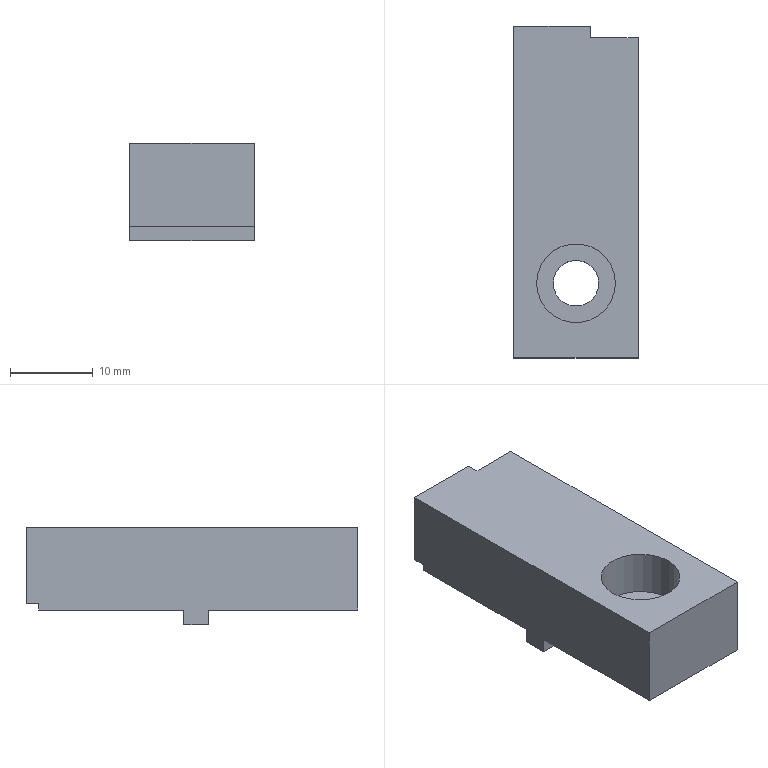Part | STEP file | Rivet push-in slide2_Default | 1 solid | 19 faces | box 15 x 40 x 11.8 mm | volume 5491 mm3 | plane 15 | cylinder 4 | commonest cylinder face diameters 5.5 x2 9.5 x2
STEP:
#1=CARTESIAN_POINT('',(0.,0.,0.));
#2=DIRECTION('',(0.,0.,1.));
#3=DIRECTION('',(1.,0.,0.));
#4=AXIS2_PLACEMENT_3D('',#1,#2,#3);
#5=CARTESIAN_POINT('',(22.25,-1.,4.5));
#6=VERTEX_POINT('',#5);
#7=CARTESIAN_POINT('',(22.25,-1.,10.));
#8=VERTEX_POINT('',#7);
#9=CARTESIAN_POINT('',(22.25,-1.,10.));
#10=DIRECTION('',(0.,0.,1.));
#11=VECTOR('',#10,1.);
#12=LINE('',#9,#11);
#13=CARTESIAN_POINT('',(17.5,-1.,10.));
#14=DIRECTION('',(0.,0.,1.));
#15=DIRECTION('',(1.,0.,0.));
#16=AXIS2_PLACEMENT_3D('',#13,#14,#15);
#17=CYLINDRICAL_SURFACE('',#16,4.75);
#18=CARTESIAN_POINT('',(6.283,0.));
#19=DIRECTION('',(0.,1.));
#20=VECTOR('',#19,1.);
#21=LINE('',#18,#20);
#22=(GEOMETRIC_REPRESENTATION_CONTEXT(2)PARAMETRIC_REPRESENTATION_CONTEXT()REPRESENTATION_CONTEXT('',''));
#23=DEFINITIONAL_REPRESENTATION('',(#21),#22);
#24=PCURVE('',#17,#23);
#25=CARTESIAN_POINT('',(17.5,-1.,10.));
#26=DIRECTION('',(0.,0.,1.));
#27=DIRECTION('',(1.,0.,0.));
#28=AXIS2_PLACEMENT_3D('',#25,#26,#27);
#29=CYLINDRICAL_SURFACE('',#28,4.75);
#30=CARTESIAN_POINT('',(0.,0.));
#31=DIRECTION('',(0.,1.));
#32=VECTOR('',#31,1.);
#33=LINE('',#30,#32);
#34=(GEOMETRIC_REPRESENTATION_CONTEXT(2)PARAMETRIC_REPRESENTATION_CONTEXT()REPRESENTATION_CONTEXT('',''));
#35=DEFINITIONAL_REPRESENTATION('',(#33),#34);
#36=PCURVE('',#29,#35);
#37=SURFACE_CURVE('',#12,(#24,#36),.PCURVE_S1.);
#38=EDGE_CURVE('',#6,#8,#37,.T.);
#39=ORIENTED_EDGE('',*,*,#38,.T.);
#40=CARTESIAN_POINT('',(12.75,-1.,10.));
#41=VERTEX_POINT('',#40);
#42=CARTESIAN_POINT('',(17.5,-1.,10.));
#43=DIRECTION('',(0.,0.,1.));
#44=DIRECTION('',(1.,0.,0.));
#45=AXIS2_PLACEMENT_3D('',#42,#43,#44);
#46=CIRCLE('',#45,4.75);
#47=CARTESIAN_POINT('',(0.,0.));
#48=DIRECTION('',(1.,0.));
#49=VECTOR('',#48,1.);
#50=LINE('',#47,#49);
#51=(GEOMETRIC_REPRESENTATION_CONTEXT(2)PARAMETRIC_REPRESENTATION_CONTEXT()REPRESENTATION_CONTEXT('',''));
#52=DEFINITIONAL_REPRESENTATION('',(#50),#51);
#53=PCURVE('',#17,#52);
#54=CARTESIAN_POINT('',(0.,30.,10.));
#55=DIRECTION('',(0.,0.,-1.));
#56=DIRECTION('',(-1.,0.,0.));
#57=AXIS2_PLACEMENT_3D('',#54,#55,#56);
#58=PLANE('',#57);
#59=CARTESIAN_POINT('',(-22.25,-31.));
#60=CARTESIAN_POINT('',(-22.25,-22.773));
#61=CARTESIAN_POINT('',(-15.125,-26.886));
#62=CARTESIAN_POINT('',(-8.,-31.));
#63=CARTESIAN_POINT('',(-15.125,-35.114));
#64=CARTESIAN_POINT('',(-22.25,-39.227));
#65=CARTESIAN_POINT('',(-22.25,-31.));
#66=(BOUNDED_CURVE()B_SPLINE_CURVE(2,(#59,#60,#61,#62,#63,#64,#65),.UNSPECIFIED.,.T.,.F.)B_SPLINE_CURVE_WITH_KNOTS((1,2,2,2,2,1),(-2.094,0.,2.094,4.189,6.283,8.378),.UNSPECIFIED.)CURVE()GEOMETRIC_REPRESENTATION_ITEM()RATIONAL_B_SPLINE_CURVE((1.,0.5,1.,0.5,1.,0.5,1.))REPRESENTATION_ITEM(''));
#67=(GEOMETRIC_REPRESENTATION_CONTEXT(2)PARAMETRIC_REPRESENTATION_CONTEXT()REPRESENTATION_CONTEXT('',''));
#68=DEFINITIONAL_REPRESENTATION('',(#66),#67);
#69=PCURVE('',#58,#68);
#70=SURFACE_CURVE('',#46,(#53,#69),.PCURVE_S1.);
#71=EDGE_CURVE('',#41,#8,#70,.T.);
#72=ORIENTED_EDGE('',*,*,#71,.F.);
#73=CARTESIAN_POINT('',(12.75,-1.,4.5));
#74=VERTEX_POINT('',#73);
#75=CARTESIAN_POINT('',(12.75,-1.,10.));
#76=DIRECTION('',(0.,0.,1.));
#77=VECTOR('',#76,1.);
#78=LINE('',#75,#77);
#79=CARTESIAN_POINT('',(3.142,0.));
#80=DIRECTION('',(0.,1.));
#81=VECTOR('',#80,1.);
#82=LINE('',#79,#81);
#83=(GEOMETRIC_REPRESENTATION_CONTEXT(2)PARAMETRIC_REPRESENTATION_CONTEXT()REPRESENTATION_CONTEXT('',''));
#84=DEFINITIONAL_REPRESENTATION('',(#82),#83);
#85=PCURVE('',#17,#84);
#86=CARTESIAN_POINT('',(3.142,0.));
#87=DIRECTION('',(0.,1.));
#88=VECTOR('',#87,1.);
#89=LINE('',#86,#88);
#90=(GEOMETRIC_REPRESENTATION_CONTEXT(2)PARAMETRIC_REPRESENTATION_CONTEXT()REPRESENTATION_CONTEXT('',''));
#91=DEFINITIONAL_REPRESENTATION('',(#89),#90);
#92=PCURVE('',#29,#91);
#93=SURFACE_CURVE('',#78,(#85,#92),.PCURVE_S1.);
#94=EDGE_CURVE('',#74,#41,#93,.T.);
#95=ORIENTED_EDGE('',*,*,#94,.F.);
#96=CARTESIAN_POINT('',(17.5,-1.,4.5));
#97=DIRECTION('',(0.,0.,1.));
#98=DIRECTION('',(1.,0.,0.));
#99=AXIS2_PLACEMENT_3D('',#96,#97,#98);
#100=CIRCLE('',#99,4.75);
#101=CARTESIAN_POINT('',(0.,-5.5));
#102=DIRECTION('',(1.,0.));
#103=VECTOR('',#102,1.);
#104=LINE('',#101,#103);
#105=(GEOMETRIC_REPRESENTATION_CONTEXT(2)PARAMETRIC_REPRESENTATION_CONTEXT()REPRESENTATION_CONTEXT('',''));
#106=DEFINITIONAL_REPRESENTATION('',(#104),#105);
#107=PCURVE('',#17,#106);
#108=CARTESIAN_POINT('',(20.25,-1.,4.5));
#109=DIRECTION('',(0.,0.,-1.));
#110=DIRECTION('',(-1.,0.,0.));
#111=AXIS2_PLACEMENT_3D('',#108,#109,#110);
#112=PLANE('',#111);
#113=CARTESIAN_POINT('',(-2.,0.));
#114=CARTESIAN_POINT('',(-2.,8.227));
#115=CARTESIAN_POINT('',(5.125,4.114));
#116=CARTESIAN_POINT('',(12.25,0.));
#117=CARTESIAN_POINT('',(5.125,-4.114));
#118=CARTESIAN_POINT('',(-2.,-8.227));
#119=CARTESIAN_POINT('',(-2.,0.));
#120=(BOUNDED_CURVE()B_SPLINE_CURVE(2,(#113,#114,#115,#116,#117,#118,#119),.UNSPECIFIED.,.T.,.F.)B_SPLINE_CURVE_WITH_KNOTS((1,2,2,2,2,1),(-2.094,0.,2.094,4.189,6.283,8.378),.UNSPECIFIED.)CURVE()GEOMETRIC_REPRESENTATION_ITEM()RATIONAL_B_SPLINE_CURVE((1.,0.5,1.,0.5,1.,0.5,1.))REPRESENTATION_ITEM(''));
#121=(GEOMETRIC_REPRESENTATION_CONTEXT(2)PARAMETRIC_REPRESENTATION_CONTEXT()REPRESENTATION_CONTEXT('',''));
#122=DEFINITIONAL_REPRESENTATION('',(#120),#121);
#123=PCURVE('',#112,#122);
#124=SURFACE_CURVE('',#100,(#107,#123),.PCURVE_S1.);
#125=EDGE_CURVE('',#74,#6,#124,.T.);
#126=ORIENTED_EDGE('',*,*,#125,.T.);
#127=EDGE_LOOP('',(#39,#72,#95,#126));
#128=FACE_BOUND('',#127,.F.);
#129=ADVANCED_FACE('',(#128),#17,.F.);
#130=CARTESIAN_POINT('',(20.25,-1.,0.));
#131=VERTEX_POINT('',#130);
#132=CARTESIAN_POINT('',(20.25,-1.,4.5));
#133=VERTEX_POINT('',#132);
#134=CARTESIAN_POINT('',(20.25,-1.,10.));
#135=DIRECTION('',(0.,0.,1.));
#136=VECTOR('',#135,1.);
#137=LINE('',#134,#136);
#138=CARTESIAN_POINT('',(17.5,-1.,10.));
#139=DIRECTION('',(0.,0.,1.));
#140=DIRECTION('',(1.,0.,0.));
#141=AXIS2_PLACEMENT_3D('',#138,#139,#140);
#142=CYLINDRICAL_SURFACE('',#141,2.75);
#143=CARTESIAN_POINT('',(6.283,0.));
#144=DIRECTION('',(0.,1.));
#145=VECTOR('',#144,1.);
#146=LINE('',#143,#145);
#147=(GEOMETRIC_REPRESENTATION_CONTEXT(2)PARAMETRIC_REPRESENTATION_CONTEXT()REPRESENTATION_CONTEXT('',''));
#148=DEFINITIONAL_REPRESENTATION('',(#146),#147);
#149=PCURVE('',#142,#148);
#150=CARTESIAN_POINT('',(17.5,-1.,10.));
#151=DIRECTION('',(0.,0.,1.));
#152=DIRECTION('',(1.,0.,0.));
#153=AXIS2_PLACEMENT_3D('',#150,#151,#152);
#154=CYLINDRICAL_SURFACE('',#153,2.75);
#155=CARTESIAN_POINT('',(0.,0.));
#156=DIRECTION('',(0.,1.));
#157=VECTOR('',#156,1.);
#158=LINE('',#155,#157);
#159=(GEOMETRIC_REPRESENTATION_CONTEXT(2)PARAMETRIC_REPRESENTATION_CONTEXT()REPRESENTATION_CONTEXT('',''));
#160=DEFINITIONAL_REPRESENTATION('',(#158),#159);
#161=PCURVE('',#154,#160);
#162=SURFACE_CURVE('',#137,(#149,#161),.PCURVE_S1.);
#163=EDGE_CURVE('',#131,#133,#162,.T.);
#164=ORIENTED_EDGE('',*,*,#163,.T.);
#165=CARTESIAN_POINT('',(14.75,-1.,4.5));
#166=VERTEX_POINT('',#165);
#167=CARTESIAN_POINT('',(17.5,-1.,4.5));
#168=DIRECTION('',(0.,0.,1.));
#169=DIRECTION('',(1.,0.,0.));
#170=AXIS2_PLACEMENT_3D('',#167,#168,#169);
#171=CIRCLE('',#170,2.75);
#172=CARTESIAN_POINT('',(0.,-5.5));
#173=DIRECTION('',(1.,0.));
#174=VECTOR('',#173,1.);
#175=LINE('',#172,#174);
#176=(GEOMETRIC_REPRESENTATION_CONTEXT(2)PARAMETRIC_REPRESENTATION_CONTEXT()REPRESENTATION_CONTEXT('',''));
#177=DEFINITIONAL_REPRESENTATION('',(#175),#176);
#178=PCURVE('',#142,#177);
#179=CARTESIAN_POINT('',(0.,0.));
#180=CARTESIAN_POINT('',(0.,4.763));
#181=CARTESIAN_POINT('',(4.125,2.382));
#182=CARTESIAN_POINT('',(8.25,0.));
#183=CARTESIAN_POINT('',(4.125,-2.382));
#184=CARTESIAN_POINT('',(0.,-4.763));
#185=CARTESIAN_POINT('',(0.,0.));
#186=(BOUNDED_CURVE()B_SPLINE_CURVE(2,(#179,#180,#181,#182,#183,#184,#185),.UNSPECIFIED.,.T.,.F.)B_SPLINE_CURVE_WITH_KNOTS((1,2,2,2,2,1),(-2.094,0.,2.094,4.189,6.283,8.378),.UNSPECIFIED.)CURVE()GEOMETRIC_REPRESENTATION_ITEM()RATIONAL_B_SPLINE_CURVE((1.,0.5,1.,0.5,1.,0.5,1.))REPRESENTATION_ITEM(''));
#187=(GEOMETRIC_REPRESENTATION_CONTEXT(2)PARAMETRIC_REPRESENTATION_CONTEXT()REPRESENTATION_CONTEXT('',''));
#188=DEFINITIONAL_REPRESENTATION('',(#186),#187);
#189=PCURVE('',#112,#188);
#190=SURFACE_CURVE('',#171,(#178,#189),.PCURVE_S1.);
#191=EDGE_CURVE('',#166,#133,#190,.T.);
#192=ORIENTED_EDGE('',*,*,#191,.F.);
#193=CARTESIAN_POINT('',(14.75,-1.,0.));
#194=VERTEX_POINT('',#193);
#195=CARTESIAN_POINT('',(14.75,-1.,10.));
#196=DIRECTION('',(0.,0.,1.));
#197=VECTOR('',#196,1.);
#198=LINE('',#195,#197);
#199=CARTESIAN_POINT('',(3.142,0.));
#200=DIRECTION('',(0.,1.));
#201=VECTOR('',#200,1.);
#202=LINE('',#199,#201);
#203=(GEOMETRIC_REPRESENTATION_CONTEXT(2)PARAMETRIC_REPRESENTATION_CONTEXT()REPRESENTATION_CONTEXT('',''));
#204=DEFINITIONAL_REPRESENTATION('',(#202),#203);
#205=PCURVE('',#142,#204);
#206=CARTESIAN_POINT('',(3.142,0.));
#207=DIRECTION('',(0.,1.));
#208=VECTOR('',#207,1.);
#209=LINE('',#206,#208);
#210=(GEOMETRIC_REPRESENTATION_CONTEXT(2)PARAMETRIC_REPRESENTATION_CONTEXT()REPRESENTATION_CONTEXT('',''));
#211=DEFINITIONAL_REPRESENTATION('',(#209),#210);
#212=PCURVE('',#154,#211);
#213=SURFACE_CURVE('',#198,(#205,#212),.PCURVE_S1.);
#214=EDGE_CURVE('',#194,#166,#213,.T.);
#215=ORIENTED_EDGE('',*,*,#214,.F.);
#216=CARTESIAN_POINT('',(17.5,-1.,0.));
#217=DIRECTION('',(0.,0.,-1.));
#218=DIRECTION('',(-1.,0.,0.));
#219=AXIS2_PLACEMENT_3D('',#216,#217,#218);
#220=CIRCLE('',#219,2.75);
#221=CARTESIAN_POINT('',(9.425,-10.));
#222=DIRECTION('',(-1.,0.));
#223=VECTOR('',#222,1.);
#224=LINE('',#221,#223);
#225=(GEOMETRIC_REPRESENTATION_CONTEXT(2)PARAMETRIC_REPRESENTATION_CONTEXT()REPRESENTATION_CONTEXT('',''));
#226=DEFINITIONAL_REPRESENTATION('',(#224),#225);
#227=PCURVE('',#142,#226);
#228=CARTESIAN_POINT('',(0.,30.,0.));
#229=DIRECTION('',(0.,0.,-1.));
#230=DIRECTION('',(-1.,0.,0.));
#231=AXIS2_PLACEMENT_3D('',#228,#229,#230);
#232=PLANE('',#231);
#233=CARTESIAN_POINT('',(-17.5,-31.));
#234=DIRECTION('',(1.,0.));
#235=AXIS2_PLACEMENT_2D('',#233,#234);
#236=CIRCLE('',#235,2.75);
#237=(GEOMETRIC_REPRESENTATION_CONTEXT(2)PARAMETRIC_REPRESENTATION_CONTEXT()REPRESENTATION_CONTEXT('',''));
#238=DEFINITIONAL_REPRESENTATION('',(#236),#237);
#239=PCURVE('',#232,#238);
#240=SURFACE_CURVE('',#220,(#227,#239),.PCURVE_S1.);
#241=EDGE_CURVE('',#131,#194,#240,.T.);
#242=ORIENTED_EDGE('',*,*,#241,.F.);
#243=EDGE_LOOP('',(#164,#192,#215,#242));
#244=FACE_BOUND('',#243,.F.);
#245=ADVANCED_FACE('',(#244),#142,.F.);
#246=CARTESIAN_POINT('',(25.,28.6,10.));
#247=VERTEX_POINT('',#246);
#248=CARTESIAN_POINT('',(25.,28.6,0.8));
#249=VERTEX_POINT('',#248);
#250=CARTESIAN_POINT('',(25.,28.6,10.));
#251=DIRECTION('',(0.,0.,-1.));
#252=VECTOR('',#251,1.);
#253=LINE('',#250,#252);
#254=CARTESIAN_POINT('',(25.,0.,10.));
#255=DIRECTION('',(-1.,0.,0.));
#256=DIRECTION('',(0.,0.,1.));
#257=AXIS2_PLACEMENT_3D('',#254,#255,#256);
#258=PLANE('',#257);
#259=CARTESIAN_POINT('',(0.,28.6));
#260=DIRECTION('',(-1.,0.));
#261=VECTOR('',#260,1.);
#262=LINE('',#259,#261);
#263=(GEOMETRIC_REPRESENTATION_CONTEXT(2)PARAMETRIC_REPRESENTATION_CONTEXT()REPRESENTATION_CONTEXT('',''));
#264=DEFINITIONAL_REPRESENTATION('',(#262),#263);
#265=PCURVE('',#258,#264);
#266=CARTESIAN_POINT('',(25.,28.6,0.8));
#267=DIRECTION('',(0.,1.,0.));
#268=DIRECTION('',(0.,0.,1.));
#269=AXIS2_PLACEMENT_3D('',#266,#267,#268);
#270=PLANE('',#269);
#271=CARTESIAN_POINT('',(9.2,0.));
#272=DIRECTION('',(-1.,0.));
#273=VECTOR('',#272,1.);
#274=LINE('',#271,#273);
#275=(GEOMETRIC_REPRESENTATION_CONTEXT(2)PARAMETRIC_REPRESENTATION_CONTEXT()REPRESENTATION_CONTEXT('',''));
#276=DEFINITIONAL_REPRESENTATION('',(#274),#275);
#277=PCURVE('',#270,#276);
#278=SURFACE_CURVE('',#253,(#265,#277),.PCURVE_S1.);
#279=EDGE_CURVE('',#247,#249,#278,.T.);
#280=ORIENTED_EDGE('',*,*,#279,.F.);
#281=CARTESIAN_POINT('',(25.,-10.,10.));
#282=VERTEX_POINT('',#281);
#283=CARTESIAN_POINT('',(25.,0.,10.));
#284=DIRECTION('',(0.,1.,0.));
#285=VECTOR('',#284,1.);
#286=LINE('',#283,#285);
#287=CARTESIAN_POINT('',(0.,0.));
#288=DIRECTION('',(0.,1.));
#289=VECTOR('',#288,1.);
#290=LINE('',#287,#289);
#291=(GEOMETRIC_REPRESENTATION_CONTEXT(2)PARAMETRIC_REPRESENTATION_CONTEXT()REPRESENTATION_CONTEXT('',''));
#292=DEFINITIONAL_REPRESENTATION('',(#290),#291);
#293=PCURVE('',#258,#292);
#294=CARTESIAN_POINT('',(-25.,-30.));
#295=DIRECTION('',(0.,1.));
#296=VECTOR('',#295,1.);
#297=LINE('',#294,#296);
#298=(GEOMETRIC_REPRESENTATION_CONTEXT(2)PARAMETRIC_REPRESENTATION_CONTEXT()REPRESENTATION_CONTEXT('',''));
#299=DEFINITIONAL_REPRESENTATION('',(#297),#298);
#300=PCURVE('',#58,#299);
#301=SURFACE_CURVE('',#286,(#293,#300),.PCURVE_S1.);
#302=EDGE_CURVE('',#282,#247,#301,.T.);
#303=ORIENTED_EDGE('',*,*,#302,.F.);
#304=CARTESIAN_POINT('',(25.,-10.,0.));
#305=VERTEX_POINT('',#304);
#306=CARTESIAN_POINT('',(25.,-10.,10.));
#307=DIRECTION('',(0.,0.,-1.));
#308=VECTOR('',#307,1.);
#309=LINE('',#306,#308);
#310=CARTESIAN_POINT('',(0.,-10.));
#311=DIRECTION('',(-1.,0.));
#312=VECTOR('',#311,1.);
#313=LINE('',#310,#312);
#314=(GEOMETRIC_REPRESENTATION_CONTEXT(2)PARAMETRIC_REPRESENTATION_CONTEXT()REPRESENTATION_CONTEXT('',''));
#315=DEFINITIONAL_REPRESENTATION('',(#313),#314);
#316=PCURVE('',#258,#315);
#317=CARTESIAN_POINT('',(0.,-10.,10.));
#318=DIRECTION('',(0.,1.,0.));
#319=DIRECTION('',(0.,0.,1.));
#320=AXIS2_PLACEMENT_3D('',#317,#318,#319);
#321=PLANE('',#320);
#322=CARTESIAN_POINT('',(0.,25.));
#323=DIRECTION('',(-1.,0.));
#324=VECTOR('',#323,1.);
#325=LINE('',#322,#324);
#326=(GEOMETRIC_REPRESENTATION_CONTEXT(2)PARAMETRIC_REPRESENTATION_CONTEXT()REPRESENTATION_CONTEXT('',''));
#327=DEFINITIONAL_REPRESENTATION('',(#325),#326);
#328=PCURVE('',#321,#327);
#329=SURFACE_CURVE('',#309,(#316,#328),.PCURVE_S1.);
#330=EDGE_CURVE('',#282,#305,#329,.T.);
#331=ORIENTED_EDGE('',*,*,#330,.T.);
#332=CARTESIAN_POINT('',(25.,8.01,0.));
#333=VERTEX_POINT('',#332);
#334=CARTESIAN_POINT('',(25.,0.,0.));
#335=DIRECTION('',(0.,1.,0.));
#336=VECTOR('',#335,1.);
#337=LINE('',#334,#336);
#338=CARTESIAN_POINT('',(-10.,0.));
#339=DIRECTION('',(0.,1.));
#340=VECTOR('',#339,1.);
#341=LINE('',#338,#340);
#342=(GEOMETRIC_REPRESENTATION_CONTEXT(2)PARAMETRIC_REPRESENTATION_CONTEXT()REPRESENTATION_CONTEXT('',''));
#343=DEFINITIONAL_REPRESENTATION('',(#341),#342);
#344=PCURVE('',#258,#343);
#345=CARTESIAN_POINT('',(-25.,-30.));
#346=DIRECTION('',(0.,1.));
#347=VECTOR('',#346,1.);
#348=LINE('',#345,#347);
#349=(GEOMETRIC_REPRESENTATION_CONTEXT(2)PARAMETRIC_REPRESENTATION_CONTEXT()REPRESENTATION_CONTEXT('',''));
#350=DEFINITIONAL_REPRESENTATION('',(#348),#349);
#351=PCURVE('',#232,#350);
#352=SURFACE_CURVE('',#337,(#344,#351),.PCURVE_S1.);
#353=EDGE_CURVE('',#305,#333,#352,.T.);
#354=ORIENTED_EDGE('',*,*,#353,.T.);
#355=CARTESIAN_POINT('',(25.,8.01,-1.8));
#356=VERTEX_POINT('',#355);
#357=CARTESIAN_POINT('',(25.,8.01,-1.8));
#358=DIRECTION('',(0.,0.,1.));
#359=VECTOR('',#358,1.);
#360=LINE('',#357,#359);
#361=CARTESIAN_POINT('',(-11.8,8.01));
#362=DIRECTION('',(1.,0.));
#363=VECTOR('',#362,1.);
#364=LINE('',#361,#363);
#365=(GEOMETRIC_REPRESENTATION_CONTEXT(2)PARAMETRIC_REPRESENTATION_CONTEXT()REPRESENTATION_CONTEXT('',''));
#366=DEFINITIONAL_REPRESENTATION('',(#364),#365);
#367=PCURVE('',#258,#366);
#368=CARTESIAN_POINT('',(0.,8.01,-1.8));
#369=DIRECTION('',(0.,1.,0.));
#370=DIRECTION('',(-1.,0.,0.));
#371=AXIS2_PLACEMENT_3D('',#368,#369,#370);
#372=PLANE('',#371);
#373=CARTESIAN_POINT('',(-25.,0.));
#374=DIRECTION('',(0.,1.));
#375=VECTOR('',#374,1.);
#376=LINE('',#373,#375);
#377=(GEOMETRIC_REPRESENTATION_CONTEXT(2)PARAMETRIC_REPRESENTATION_CONTEXT()REPRESENTATION_CONTEXT('',''));
#378=DEFINITIONAL_REPRESENTATION('',(#376),#377);
#379=PCURVE('',#372,#378);
#380=SURFACE_CURVE('',#360,(#367,#379),.PCURVE_S1.);
#381=EDGE_CURVE('',#356,#333,#380,.T.);
#382=ORIENTED_EDGE('',*,*,#381,.F.);
#383=CARTESIAN_POINT('',(25.,10.99,-1.8));
#384=VERTEX_POINT('',#383);
#385=CARTESIAN_POINT('',(25.,8.01,-1.8));
#386=DIRECTION('',(0.,-1.,0.));
#387=VECTOR('',#386,1.);
#388=LINE('',#385,#387);
#389=CARTESIAN_POINT('',(-11.8,8.01));
#390=DIRECTION('',(0.,-1.));
#391=VECTOR('',#390,1.);
#392=LINE('',#389,#391);
#393=(GEOMETRIC_REPRESENTATION_CONTEXT(2)PARAMETRIC_REPRESENTATION_CONTEXT()REPRESENTATION_CONTEXT('',''));
#394=DEFINITIONAL_REPRESENTATION('',(#392),#393);
#395=PCURVE('',#258,#394);
#396=CARTESIAN_POINT('',(0.,10.99,-1.8));
#397=DIRECTION('',(0.,0.,-1.));
#398=DIRECTION('',(-1.,0.,0.));
#399=AXIS2_PLACEMENT_3D('',#396,#397,#398);
#400=PLANE('',#399);
#401=CARTESIAN_POINT('',(-25.,-2.98));
#402=DIRECTION('',(0.,-1.));
#403=VECTOR('',#402,1.);
#404=LINE('',#401,#403);
#405=(GEOMETRIC_REPRESENTATION_CONTEXT(2)PARAMETRIC_REPRESENTATION_CONTEXT()REPRESENTATION_CONTEXT('',''));
#406=DEFINITIONAL_REPRESENTATION('',(#404),#405);
#407=PCURVE('',#400,#406);
#408=SURFACE_CURVE('',#388,(#395,#407),.PCURVE_S1.);
#409=EDGE_CURVE('',#384,#356,#408,.T.);
#410=ORIENTED_EDGE('',*,*,#409,.F.);
#411=CARTESIAN_POINT('',(25.,10.99,0.));
#412=VERTEX_POINT('',#411);
#413=CARTESIAN_POINT('',(25.,10.99,-1.8));
#414=DIRECTION('',(0.,0.,1.));
#415=VECTOR('',#414,1.);
#416=LINE('',#413,#415);
#417=CARTESIAN_POINT('',(-11.8,10.99));
#418=DIRECTION('',(1.,0.));
#419=VECTOR('',#418,1.);
#420=LINE('',#417,#419);
#421=(GEOMETRIC_REPRESENTATION_CONTEXT(2)PARAMETRIC_REPRESENTATION_CONTEXT()REPRESENTATION_CONTEXT('',''));
#422=DEFINITIONAL_REPRESENTATION('',(#420),#421);
#423=PCURVE('',#258,#422);
#424=CARTESIAN_POINT('',(0.,10.99,-1.8));
#425=DIRECTION('',(0.,-1.,0.));
#426=DIRECTION('',(1.,0.,0.));
#427=AXIS2_PLACEMENT_3D('',#424,#425,#426);
#428=PLANE('',#427);
#429=CARTESIAN_POINT('',(25.,0.));
#430=DIRECTION('',(0.,1.));
#431=VECTOR('',#430,1.);
#432=LINE('',#429,#431);
#433=(GEOMETRIC_REPRESENTATION_CONTEXT(2)PARAMETRIC_REPRESENTATION_CONTEXT()REPRESENTATION_CONTEXT('',''));
#434=DEFINITIONAL_REPRESENTATION('',(#432),#433);
#435=PCURVE('',#428,#434);
#436=SURFACE_CURVE('',#416,(#423,#435),.PCURVE_S1.);
#437=EDGE_CURVE('',#384,#412,#436,.T.);
#438=ORIENTED_EDGE('',*,*,#437,.T.);
#439=CARTESIAN_POINT('',(25.,28.5,0.));
#440=VERTEX_POINT('',#439);
#441=CARTESIAN_POINT('',(25.,0.,0.));
#442=DIRECTION('',(0.,1.,0.));
#443=VECTOR('',#442,1.);
#444=LINE('',#441,#443);
#445=CARTESIAN_POINT('',(-10.,0.));
#446=DIRECTION('',(0.,1.));
#447=VECTOR('',#446,1.);
#448=LINE('',#445,#447);
#449=(GEOMETRIC_REPRESENTATION_CONTEXT(2)PARAMETRIC_REPRESENTATION_CONTEXT()REPRESENTATION_CONTEXT('',''));
#450=DEFINITIONAL_REPRESENTATION('',(#448),#449);
#451=PCURVE('',#258,#450);
#452=CARTESIAN_POINT('',(0.,30.,0.));
#453=DIRECTION('',(0.,0.,-1.));
#454=DIRECTION('',(-1.,0.,0.));
#455=AXIS2_PLACEMENT_3D('',#452,#453,#454);
#456=PLANE('',#455);
#457=CARTESIAN_POINT('',(-25.,-30.));
#458=DIRECTION('',(0.,1.));
#459=VECTOR('',#458,1.);
#460=LINE('',#457,#459);
#461=(GEOMETRIC_REPRESENTATION_CONTEXT(2)PARAMETRIC_REPRESENTATION_CONTEXT()REPRESENTATION_CONTEXT('',''));
#462=DEFINITIONAL_REPRESENTATION('',(#460),#461);
#463=PCURVE('',#456,#462);
#464=SURFACE_CURVE('',#444,(#451,#463),.PCURVE_S1.);
#465=EDGE_CURVE('',#412,#440,#464,.T.);
#466=ORIENTED_EDGE('',*,*,#465,.T.);
#467=CARTESIAN_POINT('',(25.,28.5,0.8));
#468=VERTEX_POINT('',#467);
#469=CARTESIAN_POINT('',(25.,28.5,10.));
#470=DIRECTION('',(0.,0.,-1.));
#471=VECTOR('',#470,1.);
#472=LINE('',#469,#471);
#473=CARTESIAN_POINT('',(0.,28.5));
#474=DIRECTION('',(-1.,0.));
#475=VECTOR('',#474,1.);
#476=LINE('',#473,#475);
#477=(GEOMETRIC_REPRESENTATION_CONTEXT(2)PARAMETRIC_REPRESENTATION_CONTEXT()REPRESENTATION_CONTEXT('',''));
#478=DEFINITIONAL_REPRESENTATION('',(#476),#477);
#479=PCURVE('',#258,#478);
#480=CARTESIAN_POINT('',(-17.481,28.5,0.8));
#481=DIRECTION('',(0.,1.,0.));
#482=DIRECTION('',(0.,0.,1.));
#483=AXIS2_PLACEMENT_3D('',#480,#481,#482);
#484=PLANE('',#483);
#485=CARTESIAN_POINT('',(9.2,42.481));
#486=DIRECTION('',(-1.,0.));
#487=VECTOR('',#486,1.);
#488=LINE('',#485,#487);
#489=(GEOMETRIC_REPRESENTATION_CONTEXT(2)PARAMETRIC_REPRESENTATION_CONTEXT()REPRESENTATION_CONTEXT('',''));
#490=DEFINITIONAL_REPRESENTATION('',(#488),#489);
#491=PCURVE('',#484,#490);
#492=SURFACE_CURVE('',#472,(#479,#491),.PCURVE_S1.);
#493=EDGE_CURVE('',#468,#440,#492,.T.);
#494=ORIENTED_EDGE('',*,*,#493,.F.);
#495=CARTESIAN_POINT('',(25.,0.,0.8));
#496=DIRECTION('',(0.,1.,0.));
#497=VECTOR('',#496,1.);
#498=LINE('',#495,#497);
#499=CARTESIAN_POINT('',(-9.2,0.));
#500=DIRECTION('',(0.,1.));
#501=VECTOR('',#500,1.);
#502=LINE('',#499,#501);
#503=(GEOMETRIC_REPRESENTATION_CONTEXT(2)PARAMETRIC_REPRESENTATION_CONTEXT()REPRESENTATION_CONTEXT('',''));
#504=DEFINITIONAL_REPRESENTATION('',(#502),#503);
#505=PCURVE('',#258,#504);
#506=CARTESIAN_POINT('',(-17.481,28.5,0.8));
#507=DIRECTION('',(0.,0.,1.));
#508=DIRECTION('',(1.,0.,0.));
#509=AXIS2_PLACEMENT_3D('',#506,#507,#508);
#510=PLANE('',#509);
#511=CARTESIAN_POINT('',(42.481,-28.5));
#512=DIRECTION('',(0.,1.));
#513=VECTOR('',#512,1.);
#514=LINE('',#511,#513);
#515=(GEOMETRIC_REPRESENTATION_CONTEXT(2)PARAMETRIC_REPRESENTATION_CONTEXT()REPRESENTATION_CONTEXT('',''));
#516=DEFINITIONAL_REPRESENTATION('',(#514),#515);
#517=PCURVE('',#510,#516);
#518=SURFACE_CURVE('',#498,(#505,#517),.PCURVE_S1.);
#519=EDGE_CURVE('',#468,#249,#518,.T.);
#520=ORIENTED_EDGE('',*,*,#519,.T.);
#521=EDGE_LOOP('',(#280,#303,#331,#354,#382,#410,#438,#466,#494,#520));
#522=FACE_BOUND('',#521,.T.);
#523=ADVANCED_FACE('',(#522),#258,.F.);
#524=CARTESIAN_POINT('',(10.,28.5,0.));
#525=VERTEX_POINT('',#524);
#526=CARTESIAN_POINT('',(10.,10.99,0.));
#527=VERTEX_POINT('',#526);
#528=CARTESIAN_POINT('',(10.,30.,0.));
#529=DIRECTION('',(0.,-1.,0.));
#530=VECTOR('',#529,1.);
#531=LINE('',#528,#530);
#532=CARTESIAN_POINT('',(-10.,0.));
#533=DIRECTION('',(0.,-1.));
#534=VECTOR('',#533,1.);
#535=LINE('',#532,#534);
#536=(GEOMETRIC_REPRESENTATION_CONTEXT(2)PARAMETRIC_REPRESENTATION_CONTEXT()REPRESENTATION_CONTEXT('',''));
#537=DEFINITIONAL_REPRESENTATION('',(#535),#536);
#538=PCURVE('',#456,#537);
#539=CARTESIAN_POINT('',(10.,0.,10.));
#540=DIRECTION('',(1.,0.,0.));
#541=DIRECTION('',(0.,0.,-1.));
#542=AXIS2_PLACEMENT_3D('',#539,#540,#541);
#543=PLANE('',#542);
#544=CARTESIAN_POINT('',(10.,30.));
#545=DIRECTION('',(0.,-1.));
#546=VECTOR('',#545,1.);
#547=LINE('',#544,#546);
#548=(GEOMETRIC_REPRESENTATION_CONTEXT(2)PARAMETRIC_REPRESENTATION_CONTEXT()REPRESENTATION_CONTEXT('',''));
#549=DEFINITIONAL_REPRESENTATION('',(#547),#548);
#550=PCURVE('',#543,#549);
#551=SURFACE_CURVE('',#531,(#538,#550),.PCURVE_S1.);
#552=EDGE_CURVE('',#525,#527,#551,.T.);
#553=ORIENTED_EDGE('',*,*,#552,.F.);
#554=CARTESIAN_POINT('',(0.,28.5,0.));
#555=DIRECTION('',(1.,0.,0.));
#556=VECTOR('',#555,1.);
#557=LINE('',#554,#556);
#558=CARTESIAN_POINT('',(0.,-1.5));
#559=DIRECTION('',(-1.,0.));
#560=VECTOR('',#559,1.);
#561=LINE('',#558,#560);
#562=(GEOMETRIC_REPRESENTATION_CONTEXT(2)PARAMETRIC_REPRESENTATION_CONTEXT()REPRESENTATION_CONTEXT('',''));
#563=DEFINITIONAL_REPRESENTATION('',(#561),#562);
#564=PCURVE('',#456,#563);
#565=CARTESIAN_POINT('',(-0.8,17.481));
#566=DIRECTION('',(0.,1.));
#567=VECTOR('',#566,1.);
#568=LINE('',#565,#567);
#569=(GEOMETRIC_REPRESENTATION_CONTEXT(2)PARAMETRIC_REPRESENTATION_CONTEXT()REPRESENTATION_CONTEXT('',''));
#570=DEFINITIONAL_REPRESENTATION('',(#568),#569);
#571=PCURVE('',#484,#570);
#572=SURFACE_CURVE('',#557,(#564,#571),.PCURVE_S1.);
#573=EDGE_CURVE('',#525,#440,#572,.T.);
#574=ORIENTED_EDGE('',*,*,#573,.T.);
#575=ORIENTED_EDGE('',*,*,#465,.F.);
#576=CARTESIAN_POINT('',(0.,10.99,0.));
#577=DIRECTION('',(1.,0.,0.));
#578=VECTOR('',#577,1.);
#579=LINE('',#576,#578);
#580=CARTESIAN_POINT('',(0.,-19.01));
#581=DIRECTION('',(-1.,0.));
#582=VECTOR('',#581,1.);
#583=LINE('',#580,#582);
#584=(GEOMETRIC_REPRESENTATION_CONTEXT(2)PARAMETRIC_REPRESENTATION_CONTEXT()REPRESENTATION_CONTEXT('',''));
#585=DEFINITIONAL_REPRESENTATION('',(#583),#584);
#586=PCURVE('',#456,#585);
#587=CARTESIAN_POINT('',(0.,1.8));
#588=DIRECTION('',(1.,0.));
#589=VECTOR('',#588,1.);
#590=LINE('',#587,#589);
#591=(GEOMETRIC_REPRESENTATION_CONTEXT(2)PARAMETRIC_REPRESENTATION_CONTEXT()REPRESENTATION_CONTEXT('',''));
#592=DEFINITIONAL_REPRESENTATION('',(#590),#591);
#593=PCURVE('',#428,#592);
#594=SURFACE_CURVE('',#579,(#586,#593),.PCURVE_S1.);
#595=EDGE_CURVE('',#527,#412,#594,.T.);
#596=ORIENTED_EDGE('',*,*,#595,.F.);
#597=EDGE_LOOP('',(#553,#574,#575,#596));
#598=FACE_BOUND('',#597,.T.);
#599=ADVANCED_FACE('',(#598),#456,.T.);
#600=ORIENTED_EDGE('',*,*,#241,.F.);
#601=CARTESIAN_POINT('',(17.5,-1.,0.));
#602=DIRECTION('',(0.,0.,-1.));
#603=DIRECTION('',(-1.,0.,0.));
#604=AXIS2_PLACEMENT_3D('',#601,#602,#603);
#605=CIRCLE('',#604,2.75);
#606=CARTESIAN_POINT('',(-17.5,-31.));
#607=DIRECTION('',(1.,0.));
#608=AXIS2_PLACEMENT_2D('',#606,#607);
#609=CIRCLE('',#608,2.75);
#610=(GEOMETRIC_REPRESENTATION_CONTEXT(2)PARAMETRIC_REPRESENTATION_CONTEXT()REPRESENTATION_CONTEXT('',''));
#611=DEFINITIONAL_REPRESENTATION('',(#609),#610);
#612=PCURVE('',#232,#611);
#613=CARTESIAN_POINT('',(3.142,-10.));
#614=DIRECTION('',(-1.,0.));
#615=VECTOR('',#614,1.);
#616=LINE('',#613,#615);
#617=(GEOMETRIC_REPRESENTATION_CONTEXT(2)PARAMETRIC_REPRESENTATION_CONTEXT()REPRESENTATION_CONTEXT('',''));
#618=DEFINITIONAL_REPRESENTATION('',(#616),#617);
#619=PCURVE('',#154,#618);
#620=SURFACE_CURVE('',#605,(#612,#619),.PCURVE_S1.);
#621=EDGE_CURVE('',#194,#131,#620,.T.);
#622=ORIENTED_EDGE('',*,*,#621,.F.);
#623=EDGE_LOOP('',(#600,#622));
#624=FACE_BOUND('',#623,.T.);
#625=CARTESIAN_POINT('',(10.,8.01,0.));
#626=VERTEX_POINT('',#625);
#627=CARTESIAN_POINT('',(0.,8.01,0.));
#628=DIRECTION('',(-1.,0.,0.));
#629=VECTOR('',#628,1.);
#630=LINE('',#627,#629);
#631=CARTESIAN_POINT('',(0.,-21.99));
#632=DIRECTION('',(1.,0.));
#633=VECTOR('',#632,1.);
#634=LINE('',#631,#633);
#635=(GEOMETRIC_REPRESENTATION_CONTEXT(2)PARAMETRIC_REPRESENTATION_CONTEXT()REPRESENTATION_CONTEXT('',''));
#636=DEFINITIONAL_REPRESENTATION('',(#634),#635);
#637=PCURVE('',#232,#636);
#638=CARTESIAN_POINT('',(0.,1.8));
#639=DIRECTION('',(1.,0.));
#640=VECTOR('',#639,1.);
#641=LINE('',#638,#640);
#642=(GEOMETRIC_REPRESENTATION_CONTEXT(2)PARAMETRIC_REPRESENTATION_CONTEXT()REPRESENTATION_CONTEXT('',''));
#643=DEFINITIONAL_REPRESENTATION('',(#641),#642);
#644=PCURVE('',#372,#643);
#645=SURFACE_CURVE('',#630,(#637,#644),.PCURVE_S1.);
#646=EDGE_CURVE('',#333,#626,#645,.T.);
#647=ORIENTED_EDGE('',*,*,#646,.F.);
#648=ORIENTED_EDGE('',*,*,#353,.F.);
#649=CARTESIAN_POINT('',(10.,-10.,0.));
#650=VERTEX_POINT('',#649);
#651=CARTESIAN_POINT('',(0.,-10.,0.));
#652=DIRECTION('',(1.,0.,0.));
#653=VECTOR('',#652,1.);
#654=LINE('',#651,#653);
#655=CARTESIAN_POINT('',(0.,-40.));
#656=DIRECTION('',(-1.,0.));
#657=VECTOR('',#656,1.);
#658=LINE('',#655,#657);
#659=(GEOMETRIC_REPRESENTATION_CONTEXT(2)PARAMETRIC_REPRESENTATION_CONTEXT()REPRESENTATION_CONTEXT('',''));
#660=DEFINITIONAL_REPRESENTATION('',(#658),#659);
#661=PCURVE('',#232,#660);
#662=CARTESIAN_POINT('',(-10.,0.));
#663=DIRECTION('',(0.,1.));
#664=VECTOR('',#663,1.);
#665=LINE('',#662,#664);
#666=(GEOMETRIC_REPRESENTATION_CONTEXT(2)PARAMETRIC_REPRESENTATION_CONTEXT()REPRESENTATION_CONTEXT('',''));
#667=DEFINITIONAL_REPRESENTATION('',(#665),#666);
#668=PCURVE('',#321,#667);
#669=SURFACE_CURVE('',#654,(#661,#668),.PCURVE_S1.);
#670=EDGE_CURVE('',#650,#305,#669,.T.);
#671=ORIENTED_EDGE('',*,*,#670,.F.);
#672=CARTESIAN_POINT('',(10.,30.,0.));
#673=DIRECTION('',(0.,-1.,0.));
#674=VECTOR('',#673,1.);
#675=LINE('',#672,#674);
#676=CARTESIAN_POINT('',(-10.,0.));
#677=DIRECTION('',(0.,-1.));
#678=VECTOR('',#677,1.);
#679=LINE('',#676,#678);
#680=(GEOMETRIC_REPRESENTATION_CONTEXT(2)PARAMETRIC_REPRESENTATION_CONTEXT()REPRESENTATION_CONTEXT('',''));
#681=DEFINITIONAL_REPRESENTATION('',(#679),#680);
#682=PCURVE('',#232,#681);
#683=CARTESIAN_POINT('',(10.,30.));
#684=DIRECTION('',(0.,-1.));
#685=VECTOR('',#684,1.);
#686=LINE('',#683,#685);
#687=(GEOMETRIC_REPRESENTATION_CONTEXT(2)PARAMETRIC_REPRESENTATION_CONTEXT()REPRESENTATION_CONTEXT('',''));
#688=DEFINITIONAL_REPRESENTATION('',(#686),#687);
#689=PCURVE('',#543,#688);
#690=SURFACE_CURVE('',#675,(#682,#689),.PCURVE_S1.);
#691=EDGE_CURVE('',#626,#650,#690,.T.);
#692=ORIENTED_EDGE('',*,*,#691,.F.);
#693=EDGE_LOOP('',(#647,#648,#671,#692));
#694=FACE_BOUND('',#693,.T.);
#695=ADVANCED_FACE('',(#624,#694),#232,.T.);
#696=CARTESIAN_POINT('',(10.,30.,10.));
#697=VERTEX_POINT('',#696);
#698=CARTESIAN_POINT('',(10.,30.,0.8));
#699=VERTEX_POINT('',#698);
#700=CARTESIAN_POINT('',(10.,30.,10.));
#701=DIRECTION('',(0.,0.,-1.));
#702=VECTOR('',#701,1.);
#703=LINE('',#700,#702);
#704=CARTESIAN_POINT('',(0.,30.));
#705=DIRECTION('',(1.,0.));
#706=VECTOR('',#705,1.);
#707=LINE('',#704,#706);
#708=(GEOMETRIC_REPRESENTATION_CONTEXT(2)PARAMETRIC_REPRESENTATION_CONTEXT()REPRESENTATION_CONTEXT('',''));
#709=DEFINITIONAL_REPRESENTATION('',(#707),#708);
#710=PCURVE('',#543,#709);
#711=CARTESIAN_POINT('',(0.,30.,10.));
#712=DIRECTION('',(0.,-1.,0.));
#713=DIRECTION('',(0.,0.,-1.));
#714=AXIS2_PLACEMENT_3D('',#711,#712,#713);
#715=PLANE('',#714);
#716=CARTESIAN_POINT('',(0.,10.));
#717=DIRECTION('',(1.,0.));
#718=VECTOR('',#717,1.);
#719=LINE('',#716,#718);
#720=(GEOMETRIC_REPRESENTATION_CONTEXT(2)PARAMETRIC_REPRESENTATION_CONTEXT()REPRESENTATION_CONTEXT('',''));
#721=DEFINITIONAL_REPRESENTATION('',(#719),#720);
#722=PCURVE('',#715,#721);
#723=SURFACE_CURVE('',#703,(#710,#722),.PCURVE_S1.);
#724=EDGE_CURVE('',#697,#699,#723,.T.);
#725=ORIENTED_EDGE('',*,*,#724,.T.);
#726=CARTESIAN_POINT('',(10.,28.5,0.8));
#727=VERTEX_POINT('',#726);
#728=CARTESIAN_POINT('',(10.,0.,0.8));
#729=DIRECTION('',(0.,-1.,0.));
#730=VECTOR('',#729,1.);
#731=LINE('',#728,#730);
#732=CARTESIAN_POINT('',(9.2,0.));
#733=DIRECTION('',(0.,-1.));
#734=VECTOR('',#733,1.);
#735=LINE('',#732,#734);
#736=(GEOMETRIC_REPRESENTATION_CONTEXT(2)PARAMETRIC_REPRESENTATION_CONTEXT()REPRESENTATION_CONTEXT('',''));
#737=DEFINITIONAL_REPRESENTATION('',(#735),#736);
#738=PCURVE('',#543,#737);
#739=CARTESIAN_POINT('',(27.481,-28.5));
#740=DIRECTION('',(0.,-1.));
#741=VECTOR('',#740,1.);
#742=LINE('',#739,#741);
#743=(GEOMETRIC_REPRESENTATION_CONTEXT(2)PARAMETRIC_REPRESENTATION_CONTEXT()REPRESENTATION_CONTEXT('',''));
#744=DEFINITIONAL_REPRESENTATION('',(#742),#743);
#745=PCURVE('',#510,#744);
#746=SURFACE_CURVE('',#731,(#738,#745),.PCURVE_S1.);
#747=EDGE_CURVE('',#699,#727,#746,.T.);
#748=ORIENTED_EDGE('',*,*,#747,.T.);
#749=CARTESIAN_POINT('',(10.,28.5,10.));
#750=DIRECTION('',(0.,0.,1.));
#751=VECTOR('',#750,1.);
#752=LINE('',#749,#751);
#753=CARTESIAN_POINT('',(0.,28.5));
#754=DIRECTION('',(-1.,0.));
#755=VECTOR('',#754,1.);
#756=LINE('',#753,#755);
#757=(GEOMETRIC_REPRESENTATION_CONTEXT(2)PARAMETRIC_REPRESENTATION_CONTEXT()REPRESENTATION_CONTEXT('',''));
#758=DEFINITIONAL_REPRESENTATION('',(#756),#757);
#759=PCURVE('',#543,#758);
#760=CARTESIAN_POINT('',(9.2,27.481));
#761=DIRECTION('',(1.,0.));
#762=VECTOR('',#761,1.);
#763=LINE('',#760,#762);
#764=(GEOMETRIC_REPRESENTATION_CONTEXT(2)PARAMETRIC_REPRESENTATION_CONTEXT()REPRESENTATION_CONTEXT('',''));
#765=DEFINITIONAL_REPRESENTATION('',(#763),#764);
#766=PCURVE('',#484,#765);
#767=SURFACE_CURVE('',#752,(#759,#766),.PCURVE_S1.);
#768=EDGE_CURVE('',#525,#727,#767,.T.);
#769=ORIENTED_EDGE('',*,*,#768,.F.);
#770=ORIENTED_EDGE('',*,*,#552,.T.);
#771=CARTESIAN_POINT('',(10.,10.99,-1.8));
#772=VERTEX_POINT('',#771);
#773=CARTESIAN_POINT('',(10.,10.99,-1.8));
#774=DIRECTION('',(0.,0.,1.));
#775=VECTOR('',#774,1.);
#776=LINE('',#773,#775);
#777=CARTESIAN_POINT('',(11.8,10.99));
#778=DIRECTION('',(-1.,0.));
#779=VECTOR('',#778,1.);
#780=LINE('',#777,#779);
#781=(GEOMETRIC_REPRESENTATION_CONTEXT(2)PARAMETRIC_REPRESENTATION_CONTEXT()REPRESENTATION_CONTEXT('',''));
#782=DEFINITIONAL_REPRESENTATION('',(#780),#781);
#783=PCURVE('',#543,#782);
#784=CARTESIAN_POINT('',(10.,0.));
#785=DIRECTION('',(0.,1.));
#786=VECTOR('',#785,1.);
#787=LINE('',#784,#786);
#788=(GEOMETRIC_REPRESENTATION_CONTEXT(2)PARAMETRIC_REPRESENTATION_CONTEXT()REPRESENTATION_CONTEXT('',''));
#789=DEFINITIONAL_REPRESENTATION('',(#787),#788);
#790=PCURVE('',#428,#789);
#791=SURFACE_CURVE('',#776,(#783,#790),.PCURVE_S1.);
#792=EDGE_CURVE('',#772,#527,#791,.T.);
#793=ORIENTED_EDGE('',*,*,#792,.F.);
#794=CARTESIAN_POINT('',(10.,8.01,-1.8));
#795=VERTEX_POINT('',#794);
#796=CARTESIAN_POINT('',(10.,0.,-1.8));
#797=DIRECTION('',(0.,1.,0.));
#798=VECTOR('',#797,1.);
#799=LINE('',#796,#798);
#800=CARTESIAN_POINT('',(11.8,0.));
#801=DIRECTION('',(0.,1.));
#802=VECTOR('',#801,1.);
#803=LINE('',#800,#802);
#804=(GEOMETRIC_REPRESENTATION_CONTEXT(2)PARAMETRIC_REPRESENTATION_CONTEXT()REPRESENTATION_CONTEXT('',''));
#805=DEFINITIONAL_REPRESENTATION('',(#803),#804);
#806=PCURVE('',#543,#805);
#807=CARTESIAN_POINT('',(-10.,-10.99));
#808=DIRECTION('',(0.,1.));
#809=VECTOR('',#808,1.);
#810=LINE('',#807,#809);
#811=(GEOMETRIC_REPRESENTATION_CONTEXT(2)PARAMETRIC_REPRESENTATION_CONTEXT()REPRESENTATION_CONTEXT('',''));
#812=DEFINITIONAL_REPRESENTATION('',(#810),#811);
#813=PCURVE('',#400,#812);
#814=SURFACE_CURVE('',#799,(#806,#813),.PCURVE_S1.);
#815=EDGE_CURVE('',#795,#772,#814,.T.);
#816=ORIENTED_EDGE('',*,*,#815,.F.);
#817=CARTESIAN_POINT('',(10.,8.01,10.));
#818=DIRECTION('',(0.,0.,1.));
#819=VECTOR('',#818,1.);
#820=LINE('',#817,#819);
#821=CARTESIAN_POINT('',(0.,8.01));
#822=DIRECTION('',(-1.,0.));
#823=VECTOR('',#822,1.);
#824=LINE('',#821,#823);
#825=(GEOMETRIC_REPRESENTATION_CONTEXT(2)PARAMETRIC_REPRESENTATION_CONTEXT()REPRESENTATION_CONTEXT('',''));
#826=DEFINITIONAL_REPRESENTATION('',(#824),#825);
#827=PCURVE('',#543,#826);
#828=CARTESIAN_POINT('',(-10.,11.8));
#829=DIRECTION('',(0.,1.));
#830=VECTOR('',#829,1.);
#831=LINE('',#828,#830);
#832=(GEOMETRIC_REPRESENTATION_CONTEXT(2)PARAMETRIC_REPRESENTATION_CONTEXT()REPRESENTATION_CONTEXT('',''));
#833=DEFINITIONAL_REPRESENTATION('',(#831),#832);
#834=PCURVE('',#372,#833);
#835=SURFACE_CURVE('',#820,(#827,#834),.PCURVE_S1.);
#836=EDGE_CURVE('',#795,#626,#835,.T.);
#837=ORIENTED_EDGE('',*,*,#836,.T.);
#838=ORIENTED_EDGE('',*,*,#691,.T.);
#839=CARTESIAN_POINT('',(10.,-10.,10.));
#840=VERTEX_POINT('',#839);
#841=CARTESIAN_POINT('',(10.,-10.,10.));
#842=DIRECTION('',(0.,0.,-1.));
#843=VECTOR('',#842,1.);
#844=LINE('',#841,#843);
#845=CARTESIAN_POINT('',(0.,-10.));
#846=DIRECTION('',(1.,0.));
#847=VECTOR('',#846,1.);
#848=LINE('',#845,#847);
#849=(GEOMETRIC_REPRESENTATION_CONTEXT(2)PARAMETRIC_REPRESENTATION_CONTEXT()REPRESENTATION_CONTEXT('',''));
#850=DEFINITIONAL_REPRESENTATION('',(#848),#849);
#851=PCURVE('',#543,#850);
#852=CARTESIAN_POINT('',(0.,10.));
#853=DIRECTION('',(-1.,0.));
#854=VECTOR('',#853,1.);
#855=LINE('',#852,#854);
#856=(GEOMETRIC_REPRESENTATION_CONTEXT(2)PARAMETRIC_REPRESENTATION_CONTEXT()REPRESENTATION_CONTEXT('',''));
#857=DEFINITIONAL_REPRESENTATION('',(#855),#856);
#858=PCURVE('',#321,#857);
#859=SURFACE_CURVE('',#844,(#851,#858),.PCURVE_S1.);
#860=EDGE_CURVE('',#840,#650,#859,.T.);
#861=ORIENTED_EDGE('',*,*,#860,.F.);
#862=CARTESIAN_POINT('',(10.,30.,10.));
#863=DIRECTION('',(0.,-1.,0.));
#864=VECTOR('',#863,1.);
#865=LINE('',#862,#864);
#866=CARTESIAN_POINT('',(0.,30.));
#867=DIRECTION('',(0.,-1.));
#868=VECTOR('',#867,1.);
#869=LINE('',#866,#868);
#870=(GEOMETRIC_REPRESENTATION_CONTEXT(2)PARAMETRIC_REPRESENTATION_CONTEXT()REPRESENTATION_CONTEXT('',''));
#871=DEFINITIONAL_REPRESENTATION('',(#869),#870);
#872=PCURVE('',#543,#871);
#873=CARTESIAN_POINT('',(-10.,0.));
#874=DIRECTION('',(0.,-1.));
#875=VECTOR('',#874,1.);
#876=LINE('',#873,#875);
#877=(GEOMETRIC_REPRESENTATION_CONTEXT(2)PARAMETRIC_REPRESENTATION_CONTEXT()REPRESENTATION_CONTEXT('',''));
#878=DEFINITIONAL_REPRESENTATION('',(#876),#877);
#879=PCURVE('',#58,#878);
#880=SURFACE_CURVE('',#865,(#872,#879),.PCURVE_S1.);
#881=EDGE_CURVE('',#697,#840,#880,.T.);
#882=ORIENTED_EDGE('',*,*,#881,.F.);
#883=EDGE_LOOP('',(#725,#748,#769,#770,#793,#816,#837,#838,#861,#882));
#884=FACE_BOUND('',#883,.T.);
#885=ADVANCED_FACE('',(#884),#543,.F.);
#886=ORIENTED_EDGE('',*,*,#670,.T.);
#887=ORIENTED_EDGE('',*,*,#330,.F.);
#888=CARTESIAN_POINT('',(0.,-10.,10.));
#889=DIRECTION('',(1.,0.,0.));
#890=VECTOR('',#889,1.);
#891=LINE('',#888,#890);
#892=CARTESIAN_POINT('',(0.,0.));
#893=DIRECTION('',(0.,1.));
#894=VECTOR('',#893,1.);
#895=LINE('',#892,#894);
#896=(GEOMETRIC_REPRESENTATION_CONTEXT(2)PARAMETRIC_REPRESENTATION_CONTEXT()REPRESENTATION_CONTEXT('',''));
#897=DEFINITIONAL_REPRESENTATION('',(#895),#896);
#898=PCURVE('',#321,#897);
#899=CARTESIAN_POINT('',(0.,-40.));
#900=DIRECTION('',(-1.,0.));
#901=VECTOR('',#900,1.);
#902=LINE('',#899,#901);
#903=(GEOMETRIC_REPRESENTATION_CONTEXT(2)PARAMETRIC_REPRESENTATION_CONTEXT()REPRESENTATION_CONTEXT('',''));
#904=DEFINITIONAL_REPRESENTATION('',(#902),#903);
#905=PCURVE('',#58,#904);
#906=SURFACE_CURVE('',#891,(#898,#905),.PCURVE_S1.);
#907=EDGE_CURVE('',#840,#282,#906,.T.);
#908=ORIENTED_EDGE('',*,*,#907,.F.);
#909=ORIENTED_EDGE('',*,*,#860,.T.);
#910=EDGE_LOOP('',(#886,#887,#908,#909));
#911=FACE_BOUND('',#910,.T.);
#912=ADVANCED_FACE('',(#911),#321,.F.);
#913=CARTESIAN_POINT('',(19.22,30.,10.));
#914=VERTEX_POINT('',#913);
#915=CARTESIAN_POINT('',(0.,30.,10.));
#916=DIRECTION('',(-1.,0.,0.));
#917=VECTOR('',#916,1.);
#918=LINE('',#915,#917);
#919=CARTESIAN_POINT('',(0.,0.));
#920=DIRECTION('',(0.,-1.));
#921=VECTOR('',#920,1.);
#922=LINE('',#919,#921);
#923=(GEOMETRIC_REPRESENTATION_CONTEXT(2)PARAMETRIC_REPRESENTATION_CONTEXT()REPRESENTATION_CONTEXT('',''));
#924=DEFINITIONAL_REPRESENTATION('',(#922),#923);
#925=PCURVE('',#715,#924);
#926=CARTESIAN_POINT('',(0.,0.));
#927=DIRECTION('',(1.,0.));
#928=VECTOR('',#927,1.);
#929=LINE('',#926,#928);
#930=(GEOMETRIC_REPRESENTATION_CONTEXT(2)PARAMETRIC_REPRESENTATION_CONTEXT()REPRESENTATION_CONTEXT('',''));
#931=DEFINITIONAL_REPRESENTATION('',(#929),#930);
#932=PCURVE('',#58,#931);
#933=SURFACE_CURVE('',#918,(#925,#932),.PCURVE_S1.);
#934=EDGE_CURVE('',#914,#697,#933,.T.);
#935=ORIENTED_EDGE('',*,*,#934,.F.);
#936=CARTESIAN_POINT('',(19.22,30.,0.8));
#937=VERTEX_POINT('',#936);
#938=CARTESIAN_POINT('',(19.22,30.,10.));
#939=DIRECTION('',(0.,0.,1.));
#940=VECTOR('',#939,1.);
#941=LINE('',#938,#940);
#942=CARTESIAN_POINT('',(0.,19.22));
#943=DIRECTION('',(-1.,0.));
#944=VECTOR('',#943,1.);
#945=LINE('',#942,#944);
#946=(GEOMETRIC_REPRESENTATION_CONTEXT(2)PARAMETRIC_REPRESENTATION_CONTEXT()REPRESENTATION_CONTEXT('',''));
#947=DEFINITIONAL_REPRESENTATION('',(#945),#946);
#948=PCURVE('',#715,#947);
#949=CARTESIAN_POINT('',(19.22,28.6,10.));
#950=DIRECTION('',(-1.,0.,0.));
#951=DIRECTION('',(0.,0.,1.));
#952=AXIS2_PLACEMENT_3D('',#949,#950,#951);
#953=PLANE('',#952);
#954=CARTESIAN_POINT('',(0.,1.4));
#955=DIRECTION('',(1.,0.));
#956=VECTOR('',#955,1.);
#957=LINE('',#954,#956);
#958=(GEOMETRIC_REPRESENTATION_CONTEXT(2)PARAMETRIC_REPRESENTATION_CONTEXT()REPRESENTATION_CONTEXT('',''));
#959=DEFINITIONAL_REPRESENTATION('',(#957),#958);
#960=PCURVE('',#953,#959);
#961=SURFACE_CURVE('',#941,(#948,#960),.PCURVE_S1.);
#962=EDGE_CURVE('',#937,#914,#961,.T.);
#963=ORIENTED_EDGE('',*,*,#962,.F.);
#964=CARTESIAN_POINT('',(-17.481,30.,0.8));
#965=DIRECTION('',(1.,0.,0.));
#966=VECTOR('',#965,1.);
#967=LINE('',#964,#966);
#968=CARTESIAN_POINT('',(9.2,-17.481));
#969=DIRECTION('',(0.,1.));
#970=VECTOR('',#969,1.);
#971=LINE('',#968,#970);
#972=(GEOMETRIC_REPRESENTATION_CONTEXT(2)PARAMETRIC_REPRESENTATION_CONTEXT()REPRESENTATION_CONTEXT('',''));
#973=DEFINITIONAL_REPRESENTATION('',(#971),#972);
#974=PCURVE('',#715,#973);
#975=CARTESIAN_POINT('',(0.,1.5));
#976=DIRECTION('',(1.,0.));
#977=VECTOR('',#976,1.);
#978=LINE('',#975,#977);
#979=(GEOMETRIC_REPRESENTATION_CONTEXT(2)PARAMETRIC_REPRESENTATION_CONTEXT()REPRESENTATION_CONTEXT('',''));
#980=DEFINITIONAL_REPRESENTATION('',(#978),#979);
#981=PCURVE('',#510,#980);
#982=SURFACE_CURVE('',#967,(#974,#981),.PCURVE_S1.);
#983=EDGE_CURVE('',#699,#937,#982,.T.);
#984=ORIENTED_EDGE('',*,*,#983,.F.);
#985=ORIENTED_EDGE('',*,*,#724,.F.);
#986=EDGE_LOOP('',(#935,#963,#984,#985));
#987=FACE_BOUND('',#986,.T.);
#988=ADVANCED_FACE('',(#987),#715,.F.);
#989=CARTESIAN_POINT('',(17.5,-1.,10.));
#990=DIRECTION('',(0.,0.,1.));
#991=DIRECTION('',(1.,0.,0.));
#992=AXIS2_PLACEMENT_3D('',#989,#990,#991);
#993=CIRCLE('',#992,4.75);
#994=CARTESIAN_POINT('',(-22.25,-31.));
#995=CARTESIAN_POINT('',(-22.25,-22.773));
#996=CARTESIAN_POINT('',(-15.125,-26.886));
#997=CARTESIAN_POINT('',(-8.,-31.));
#998=CARTESIAN_POINT('',(-15.125,-35.114));
#999=CARTESIAN_POINT('',(-22.25,-39.227));
#1000=CARTESIAN_POINT('',(-22.25,-31.));
#1001=(BOUNDED_CURVE()B_SPLINE_CURVE(2,(#994,#995,#996,#997,#998,#999,#1000),.UNSPECIFIED.,.T.,.F.)B_SPLINE_CURVE_WITH_KNOTS((1,2,2,2,2,1),(-2.094,0.,2.094,4.189,6.283,8.378),.UNSPECIFIED.)CURVE()GEOMETRIC_REPRESENTATION_ITEM()RATIONAL_B_SPLINE_CURVE((1.,0.5,1.,0.5,1.,0.5,1.))REPRESENTATION_ITEM(''));
#1002=(GEOMETRIC_REPRESENTATION_CONTEXT(2)PARAMETRIC_REPRESENTATION_CONTEXT()REPRESENTATION_CONTEXT('',''));
#1003=DEFINITIONAL_REPRESENTATION('',(#1001),#1002);
#1004=PCURVE('',#58,#1003);
#1005=CARTESIAN_POINT('',(0.,0.));
#1006=DIRECTION('',(1.,0.));
#1007=VECTOR('',#1006,1.);
#1008=LINE('',#1005,#1007);
#1009=(GEOMETRIC_REPRESENTATION_CONTEXT(2)PARAMETRIC_REPRESENTATION_CONTEXT()REPRESENTATION_CONTEXT('',''));
#1010=DEFINITIONAL_REPRESENTATION('',(#1008),#1009);
#1011=PCURVE('',#29,#1010);
#1012=SURFACE_CURVE('',#993,(#1004,#1011),.PCURVE_S1.);
#1013=EDGE_CURVE('',#8,#41,#1012,.T.);
#1014=ORIENTED_EDGE('',*,*,#1013,.F.);
#1015=ORIENTED_EDGE('',*,*,#71,.F.);
#1016=EDGE_LOOP('',(#1014,#1015));
#1017=FACE_BOUND('',#1016,.T.);
#1018=CARTESIAN_POINT('',(19.22,28.6,10.));
#1019=VERTEX_POINT('',#1018);
#1020=CARTESIAN_POINT('',(25.,28.6,10.));
#1021=DIRECTION('',(1.,0.,0.));
#1022=VECTOR('',#1021,1.);
#1023=LINE('',#1020,#1022);
#1024=CARTESIAN_POINT('',(-25.,-1.4));
#1025=DIRECTION('',(-1.,0.));
#1026=VECTOR('',#1025,1.);
#1027=LINE('',#1024,#1026);
#1028=(GEOMETRIC_REPRESENTATION_CONTEXT(2)PARAMETRIC_REPRESENTATION_CONTEXT()REPRESENTATION_CONTEXT('',''));
#1029=DEFINITIONAL_REPRESENTATION('',(#1027),#1028);
#1030=PCURVE('',#58,#1029);
#1031=CARTESIAN_POINT('',(9.2,0.));
#1032=DIRECTION('',(0.,1.));
#1033=VECTOR('',#1032,1.);
#1034=LINE('',#1031,#1033);
#1035=(GEOMETRIC_REPRESENTATION_CONTEXT(2)PARAMETRIC_REPRESENTATION_CONTEXT()REPRESENTATION_CONTEXT('',''));
#1036=DEFINITIONAL_REPRESENTATION('',(#1034),#1035);
#1037=PCURVE('',#270,#1036);
#1038=SURFACE_CURVE('',#1023,(#1030,#1037),.PCURVE_S1.);
#1039=EDGE_CURVE('',#1019,#247,#1038,.T.);
#1040=ORIENTED_EDGE('',*,*,#1039,.F.);
#1041=CARTESIAN_POINT('',(19.22,28.6,10.));
#1042=DIRECTION('',(0.,1.,0.));
#1043=VECTOR('',#1042,1.);
#1044=LINE('',#1041,#1043);
#1045=CARTESIAN_POINT('',(-19.22,-1.4));
#1046=DIRECTION('',(0.,1.));
#1047=VECTOR('',#1046,1.);
#1048=LINE('',#1045,#1047);
#1049=(GEOMETRIC_REPRESENTATION_CONTEXT(2)PARAMETRIC_REPRESENTATION_CONTEXT()REPRESENTATION_CONTEXT('',''));
#1050=DEFINITIONAL_REPRESENTATION('',(#1048),#1049);
#1051=PCURVE('',#58,#1050);
#1052=CARTESIAN_POINT('',(0.,0.));
#1053=DIRECTION('',(0.,1.));
#1054=VECTOR('',#1053,1.);
#1055=LINE('',#1052,#1054);
#1056=(GEOMETRIC_REPRESENTATION_CONTEXT(2)PARAMETRIC_REPRESENTATION_CONTEXT()REPRESENTATION_CONTEXT('',''));
#1057=DEFINITIONAL_REPRESENTATION('',(#1055),#1056);
#1058=PCURVE('',#953,#1057);
#1059=SURFACE_CURVE('',#1044,(#1051,#1058),.PCURVE_S1.);
#1060=EDGE_CURVE('',#1019,#914,#1059,.T.);
#1061=ORIENTED_EDGE('',*,*,#1060,.T.);
#1062=ORIENTED_EDGE('',*,*,#934,.T.);
#1063=ORIENTED_EDGE('',*,*,#881,.T.);
#1064=ORIENTED_EDGE('',*,*,#907,.T.);
#1065=ORIENTED_EDGE('',*,*,#302,.T.);
#1066=EDGE_LOOP('',(#1040,#1061,#1062,#1063,#1064,#1065));
#1067=FACE_BOUND('',#1066,.T.);
#1068=ADVANCED_FACE('',(#1017,#1067),#58,.F.);
#1069=ORIENTED_EDGE('',*,*,#595,.T.);
#1070=ORIENTED_EDGE('',*,*,#437,.F.);
#1071=CARTESIAN_POINT('',(0.,10.99,-1.8));
#1072=DIRECTION('',(1.,0.,0.));
#1073=VECTOR('',#1072,1.);
#1074=LINE('',#1071,#1073);
#1075=CARTESIAN_POINT('',(0.,0.));
#1076=DIRECTION('',(1.,0.));
#1077=VECTOR('',#1076,1.);
#1078=LINE('',#1075,#1077);
#1079=(GEOMETRIC_REPRESENTATION_CONTEXT(2)PARAMETRIC_REPRESENTATION_CONTEXT()REPRESENTATION_CONTEXT('',''));
#1080=DEFINITIONAL_REPRESENTATION('',(#1078),#1079);
#1081=PCURVE('',#428,#1080);
#1082=CARTESIAN_POINT('',(0.,0.));
#1083=DIRECTION('',(-1.,0.));
#1084=VECTOR('',#1083,1.);
#1085=LINE('',#1082,#1084);
#1086=(GEOMETRIC_REPRESENTATION_CONTEXT(2)PARAMETRIC_REPRESENTATION_CONTEXT()REPRESENTATION_CONTEXT('',''));
#1087=DEFINITIONAL_REPRESENTATION('',(#1085),#1086);
#1088=PCURVE('',#400,#1087);
#1089=SURFACE_CURVE('',#1074,(#1081,#1088),.PCURVE_S1.);
#1090=EDGE_CURVE('',#772,#384,#1089,.T.);
#1091=ORIENTED_EDGE('',*,*,#1090,.F.);
#1092=ORIENTED_EDGE('',*,*,#792,.T.);
#1093=EDGE_LOOP('',(#1069,#1070,#1091,#1092));
#1094=FACE_BOUND('',#1093,.T.);
#1095=ADVANCED_FACE('',(#1094),#428,.F.);
#1096=ORIENTED_EDGE('',*,*,#646,.T.);
#1097=ORIENTED_EDGE('',*,*,#836,.F.);
#1098=CARTESIAN_POINT('',(0.,8.01,-1.8));
#1099=DIRECTION('',(-1.,0.,0.));
#1100=VECTOR('',#1099,1.);
#1101=LINE('',#1098,#1100);
#1102=CARTESIAN_POINT('',(0.,0.));
#1103=DIRECTION('',(1.,0.));
#1104=VECTOR('',#1103,1.);
#1105=LINE('',#1102,#1104);
#1106=(GEOMETRIC_REPRESENTATION_CONTEXT(2)PARAMETRIC_REPRESENTATION_CONTEXT()REPRESENTATION_CONTEXT('',''));
#1107=DEFINITIONAL_REPRESENTATION('',(#1105),#1106);
#1108=PCURVE('',#372,#1107);
#1109=CARTESIAN_POINT('',(0.,-2.98));
#1110=DIRECTION('',(1.,0.));
#1111=VECTOR('',#1110,1.);
#1112=LINE('',#1109,#1111);
#1113=(GEOMETRIC_REPRESENTATION_CONTEXT(2)PARAMETRIC_REPRESENTATION_CONTEXT()REPRESENTATION_CONTEXT('',''));
#1114=DEFINITIONAL_REPRESENTATION('',(#1112),#1113);
#1115=PCURVE('',#400,#1114);
#1116=SURFACE_CURVE('',#1101,(#1108,#1115),.PCURVE_S1.);
#1117=EDGE_CURVE('',#356,#795,#1116,.T.);
#1118=ORIENTED_EDGE('',*,*,#1117,.F.);
#1119=ORIENTED_EDGE('',*,*,#381,.T.);
#1120=EDGE_LOOP('',(#1096,#1097,#1118,#1119));
#1121=FACE_BOUND('',#1120,.T.);
#1122=ADVANCED_FACE('',(#1121),#372,.F.);
#1123=ORIENTED_EDGE('',*,*,#815,.T.);
#1124=ORIENTED_EDGE('',*,*,#1090,.T.);
#1125=ORIENTED_EDGE('',*,*,#409,.T.);
#1126=ORIENTED_EDGE('',*,*,#1117,.T.);
#1127=EDGE_LOOP('',(#1123,#1124,#1125,#1126));
#1128=FACE_BOUND('',#1127,.T.);
#1129=ADVANCED_FACE('',(#1128),#400,.T.);
#1130=ORIENTED_EDGE('',*,*,#983,.T.);
#1131=CARTESIAN_POINT('',(19.22,28.6,0.8));
#1132=VERTEX_POINT('',#1131);
#1133=CARTESIAN_POINT('',(19.22,28.6,0.8));
#1134=DIRECTION('',(0.,1.,0.));
#1135=VECTOR('',#1134,1.);
#1136=LINE('',#1133,#1135);
#1137=CARTESIAN_POINT('',(36.701,0.1));
#1138=DIRECTION('',(0.,1.));
#1139=VECTOR('',#1138,1.);
#1140=LINE('',#1137,#1139);
#1141=(GEOMETRIC_REPRESENTATION_CONTEXT(2)PARAMETRIC_REPRESENTATION_CONTEXT()REPRESENTATION_CONTEXT('',''));
#1142=DEFINITIONAL_REPRESENTATION('',(#1140),#1141);
#1143=PCURVE('',#510,#1142);
#1144=CARTESIAN_POINT('',(-9.2,0.));
#1145=DIRECTION('',(0.,1.));
#1146=VECTOR('',#1145,1.);
#1147=LINE('',#1144,#1146);
#1148=(GEOMETRIC_REPRESENTATION_CONTEXT(2)PARAMETRIC_REPRESENTATION_CONTEXT()REPRESENTATION_CONTEXT('',''));
#1149=DEFINITIONAL_REPRESENTATION('',(#1147),#1148);
#1150=PCURVE('',#953,#1149);
#1151=SURFACE_CURVE('',#1136,(#1143,#1150),.PCURVE_S1.);
#1152=EDGE_CURVE('',#1132,#937,#1151,.T.);
#1153=ORIENTED_EDGE('',*,*,#1152,.F.);
#1154=CARTESIAN_POINT('',(25.,28.6,0.8));
#1155=DIRECTION('',(-1.,0.,0.));
#1156=VECTOR('',#1155,1.);
#1157=LINE('',#1154,#1156);
#1158=CARTESIAN_POINT('',(42.481,0.1));
#1159=DIRECTION('',(-1.,0.));
#1160=VECTOR('',#1159,1.);
#1161=LINE('',#1158,#1160);
#1162=(GEOMETRIC_REPRESENTATION_CONTEXT(2)PARAMETRIC_REPRESENTATION_CONTEXT()REPRESENTATION_CONTEXT('',''));
#1163=DEFINITIONAL_REPRESENTATION('',(#1161),#1162);
#1164=PCURVE('',#510,#1163);
#1165=CARTESIAN_POINT('',(0.,0.));
#1166=DIRECTION('',(0.,-1.));
#1167=VECTOR('',#1166,1.);
#1168=LINE('',#1165,#1167);
#1169=(GEOMETRIC_REPRESENTATION_CONTEXT(2)PARAMETRIC_REPRESENTATION_CONTEXT()REPRESENTATION_CONTEXT('',''));
#1170=DEFINITIONAL_REPRESENTATION('',(#1168),#1169);
#1171=PCURVE('',#270,#1170);
#1172=SURFACE_CURVE('',#1157,(#1164,#1171),.PCURVE_S1.);
#1173=EDGE_CURVE('',#249,#1132,#1172,.T.);
#1174=ORIENTED_EDGE('',*,*,#1173,.F.);
#1175=ORIENTED_EDGE('',*,*,#519,.F.);
#1176=CARTESIAN_POINT('',(-17.481,28.5,0.8));
#1177=DIRECTION('',(1.,0.,0.));
#1178=VECTOR('',#1177,1.);
#1179=LINE('',#1176,#1178);
#1180=CARTESIAN_POINT('',(0.,0.));
#1181=DIRECTION('',(1.,0.));
#1182=VECTOR('',#1181,1.);
#1183=LINE('',#1180,#1182);
#1184=(GEOMETRIC_REPRESENTATION_CONTEXT(2)PARAMETRIC_REPRESENTATION_CONTEXT()REPRESENTATION_CONTEXT('',''));
#1185=DEFINITIONAL_REPRESENTATION('',(#1183),#1184);
#1186=PCURVE('',#510,#1185);
#1187=CARTESIAN_POINT('',(0.,0.));
#1188=DIRECTION('',(0.,1.));
#1189=VECTOR('',#1188,1.);
#1190=LINE('',#1187,#1189);
#1191=(GEOMETRIC_REPRESENTATION_CONTEXT(2)PARAMETRIC_REPRESENTATION_CONTEXT()REPRESENTATION_CONTEXT('',''));
#1192=DEFINITIONAL_REPRESENTATION('',(#1190),#1191);
#1193=PCURVE('',#484,#1192);
#1194=SURFACE_CURVE('',#1179,(#1186,#1193),.PCURVE_S1.);
#1195=EDGE_CURVE('',#727,#468,#1194,.T.);
#1196=ORIENTED_EDGE('',*,*,#1195,.F.);
#1197=ORIENTED_EDGE('',*,*,#747,.F.);
#1198=EDGE_LOOP('',(#1130,#1153,#1174,#1175,#1196,#1197));
#1199=FACE_BOUND('',#1198,.T.);
#1200=ADVANCED_FACE('',(#1199),#510,.F.);
#1201=ORIENTED_EDGE('',*,*,#768,.T.);
#1202=ORIENTED_EDGE('',*,*,#1195,.T.);
#1203=ORIENTED_EDGE('',*,*,#493,.T.);
#1204=ORIENTED_EDGE('',*,*,#573,.F.);
#1205=EDGE_LOOP('',(#1201,#1202,#1203,#1204));
#1206=FACE_BOUND('',#1205,.T.);
#1207=ADVANCED_FACE('',(#1206),#484,.T.);
#1208=ORIENTED_EDGE('',*,*,#962,.T.);
#1209=ORIENTED_EDGE('',*,*,#1060,.F.);
#1210=CARTESIAN_POINT('',(19.22,28.6,10.));
#1211=DIRECTION('',(0.,0.,1.));
#1212=VECTOR('',#1211,1.);
#1213=LINE('',#1210,#1212);
#1214=CARTESIAN_POINT('',(0.,0.));
#1215=DIRECTION('',(1.,0.));
#1216=VECTOR('',#1215,1.);
#1217=LINE('',#1214,#1216);
#1218=(GEOMETRIC_REPRESENTATION_CONTEXT(2)PARAMETRIC_REPRESENTATION_CONTEXT()REPRESENTATION_CONTEXT('',''));
#1219=DEFINITIONAL_REPRESENTATION('',(#1217),#1218);
#1220=PCURVE('',#953,#1219);
#1221=CARTESIAN_POINT('',(9.2,-5.78));
#1222=DIRECTION('',(1.,0.));
#1223=VECTOR('',#1222,1.);
#1224=LINE('',#1221,#1223);
#1225=(GEOMETRIC_REPRESENTATION_CONTEXT(2)PARAMETRIC_REPRESENTATION_CONTEXT()REPRESENTATION_CONTEXT('',''));
#1226=DEFINITIONAL_REPRESENTATION('',(#1224),#1225);
#1227=PCURVE('',#270,#1226);
#1228=SURFACE_CURVE('',#1213,(#1220,#1227),.PCURVE_S1.);
#1229=EDGE_CURVE('',#1132,#1019,#1228,.T.);
#1230=ORIENTED_EDGE('',*,*,#1229,.F.);
#1231=ORIENTED_EDGE('',*,*,#1152,.T.);
#1232=EDGE_LOOP('',(#1208,#1209,#1230,#1231));
#1233=FACE_BOUND('',#1232,.T.);
#1234=ADVANCED_FACE('',(#1233),#953,.F.);
#1235=ORIENTED_EDGE('',*,*,#279,.T.);
#1236=ORIENTED_EDGE('',*,*,#1173,.T.);
#1237=ORIENTED_EDGE('',*,*,#1229,.T.);
#1238=ORIENTED_EDGE('',*,*,#1039,.T.);
#1239=EDGE_LOOP('',(#1235,#1236,#1237,#1238));
#1240=FACE_BOUND('',#1239,.T.);
#1241=ADVANCED_FACE('',(#1240),#270,.T.);
#1242=CARTESIAN_POINT('',(17.5,-1.,4.5));
#1243=DIRECTION('',(0.,0.,1.));
#1244=DIRECTION('',(1.,0.,0.));
#1245=AXIS2_PLACEMENT_3D('',#1242,#1243,#1244);
#1246=CIRCLE('',#1245,2.75);
#1247=CARTESIAN_POINT('',(0.,-5.5));
#1248=DIRECTION('',(1.,0.));
#1249=VECTOR('',#1248,1.);
#1250=LINE('',#1247,#1249);
#1251=(GEOMETRIC_REPRESENTATION_CONTEXT(2)PARAMETRIC_REPRESENTATION_CONTEXT()REPRESENTATION_CONTEXT('',''));
#1252=DEFINITIONAL_REPRESENTATION('',(#1250),#1251);
#1253=PCURVE('',#154,#1252);
#1254=CARTESIAN_POINT('',(0.,0.));
#1255=CARTESIAN_POINT('',(0.,4.763));
#1256=CARTESIAN_POINT('',(4.125,2.382));
#1257=CARTESIAN_POINT('',(8.25,0.));
#1258=CARTESIAN_POINT('',(4.125,-2.382));
#1259=CARTESIAN_POINT('',(0.,-4.763));
#1260=CARTESIAN_POINT('',(0.,0.));
#1261=(BOUNDED_CURVE()B_SPLINE_CURVE(2,(#1254,#1255,#1256,#1257,#1258,#1259,#1260),.UNSPECIFIED.,.T.,.F.)B_SPLINE_CURVE_WITH_KNOTS((1,2,2,2,2,1),(-2.094,0.,2.094,4.189,6.283,8.378),.UNSPECIFIED.)CURVE()GEOMETRIC_REPRESENTATION_ITEM()RATIONAL_B_SPLINE_CURVE((1.,0.5,1.,0.5,1.,0.5,1.))REPRESENTATION_ITEM(''));
#1262=(GEOMETRIC_REPRESENTATION_CONTEXT(2)PARAMETRIC_REPRESENTATION_CONTEXT()REPRESENTATION_CONTEXT('',''));
#1263=DEFINITIONAL_REPRESENTATION('',(#1261),#1262);
#1264=PCURVE('',#112,#1263);
#1265=SURFACE_CURVE('',#1246,(#1253,#1264),.PCURVE_S1.);
#1266=EDGE_CURVE('',#133,#166,#1265,.T.);
#1267=ORIENTED_EDGE('',*,*,#1266,.F.);
#1268=ORIENTED_EDGE('',*,*,#163,.F.);
#1269=ORIENTED_EDGE('',*,*,#621,.F.);
#1270=ORIENTED_EDGE('',*,*,#214,.T.);
#1271=EDGE_LOOP('',(#1267,#1268,#1269,#1270));
#1272=FACE_BOUND('',#1271,.F.);
#1273=ADVANCED_FACE('',(#1272),#154,.F.);
#1274=ORIENTED_EDGE('',*,*,#1266,.F.);
#1275=ORIENTED_EDGE('',*,*,#191,.F.);
#1276=EDGE_LOOP('',(#1274,#1275));
#1277=FACE_BOUND('',#1276,.T.);
#1278=CARTESIAN_POINT('',(17.5,-1.,4.5));
#1279=DIRECTION('',(0.,0.,1.));
#1280=DIRECTION('',(1.,0.,0.));
#1281=AXIS2_PLACEMENT_3D('',#1278,#1279,#1280);
#1282=CIRCLE('',#1281,4.75);
#1283=CARTESIAN_POINT('',(-2.,0.));
#1284=CARTESIAN_POINT('',(-2.,8.227));
#1285=CARTESIAN_POINT('',(5.125,4.114));
#1286=CARTESIAN_POINT('',(12.25,0.));
#1287=CARTESIAN_POINT('',(5.125,-4.114));
#1288=CARTESIAN_POINT('',(-2.,-8.227));
#1289=CARTESIAN_POINT('',(-2.,0.));
#1290=(BOUNDED_CURVE()B_SPLINE_CURVE(2,(#1283,#1284,#1285,#1286,#1287,#1288,#1289),.UNSPECIFIED.,.T.,.F.)B_SPLINE_CURVE_WITH_KNOTS((1,2,2,2,2,1),(-2.094,0.,2.094,4.189,6.283,8.378),.UNSPECIFIED.)CURVE()GEOMETRIC_REPRESENTATION_ITEM()RATIONAL_B_SPLINE_CURVE((1.,0.5,1.,0.5,1.,0.5,1.))REPRESENTATION_ITEM(''));
#1291=(GEOMETRIC_REPRESENTATION_CONTEXT(2)PARAMETRIC_REPRESENTATION_CONTEXT()REPRESENTATION_CONTEXT('',''));
#1292=DEFINITIONAL_REPRESENTATION('',(#1290),#1291);
#1293=PCURVE('',#112,#1292);
#1294=CARTESIAN_POINT('',(0.,-5.5));
#1295=DIRECTION('',(1.,0.));
#1296=VECTOR('',#1295,1.);
#1297=LINE('',#1294,#1296);
#1298=(GEOMETRIC_REPRESENTATION_CONTEXT(2)PARAMETRIC_REPRESENTATION_CONTEXT()REPRESENTATION_CONTEXT('',''));
#1299=DEFINITIONAL_REPRESENTATION('',(#1297),#1298);
#1300=PCURVE('',#29,#1299);
#1301=SURFACE_CURVE('',#1282,(#1293,#1300),.PCURVE_S1.);
#1302=EDGE_CURVE('',#6,#74,#1301,.T.);
#1303=ORIENTED_EDGE('',*,*,#1302,.T.);
#1304=ORIENTED_EDGE('',*,*,#125,.T.);
#1305=EDGE_LOOP('',(#1303,#1304));
#1306=FACE_BOUND('',#1305,.T.);
#1307=ADVANCED_FACE('',(#1277,#1306),#112,.F.);
#1308=ORIENTED_EDGE('',*,*,#1013,.F.);
#1309=ORIENTED_EDGE('',*,*,#38,.F.);
#1310=ORIENTED_EDGE('',*,*,#1302,.T.);
#1311=ORIENTED_EDGE('',*,*,#94,.T.);
#1312=EDGE_LOOP('',(#1308,#1309,#1310,#1311));
#1313=FACE_BOUND('',#1312,.F.);
#1314=ADVANCED_FACE('',(#1313),#29,.F.);
#1315=CLOSED_SHELL('',(#129,#245,#523,#599,#695,#885,#912,#988,#1068,#1095,#1122,#1129,#1200,#1207,#1234,#1241,#1273,#1307,#1314));
#1316=MANIFOLD_SOLID_BREP('',#1315);
#1317=(LENGTH_UNIT()NAMED_UNIT(*)SI_UNIT(.MILLI.,.METRE.));
#1318=UNCERTAINTY_MEASURE_WITH_UNIT(LENGTH_MEASURE(0.0000001),#1317,'','');
#1319=(NAMED_UNIT(*)PLANE_ANGLE_UNIT()SI_UNIT($,.RADIAN.));
#1320=(NAMED_UNIT(*)SI_UNIT($,.STERADIAN.)SOLID_ANGLE_UNIT());
#1321=(GEOMETRIC_REPRESENTATION_CONTEXT(3)GLOBAL_UNCERTAINTY_ASSIGNED_CONTEXT((#1318))GLOBAL_UNIT_ASSIGNED_CONTEXT((#1317,#1319,#1320))REPRESENTATION_CONTEXT('',''));
#1322=ADVANCED_BREP_SHAPE_REPRESENTATION('',(#4,#1316),#1321);